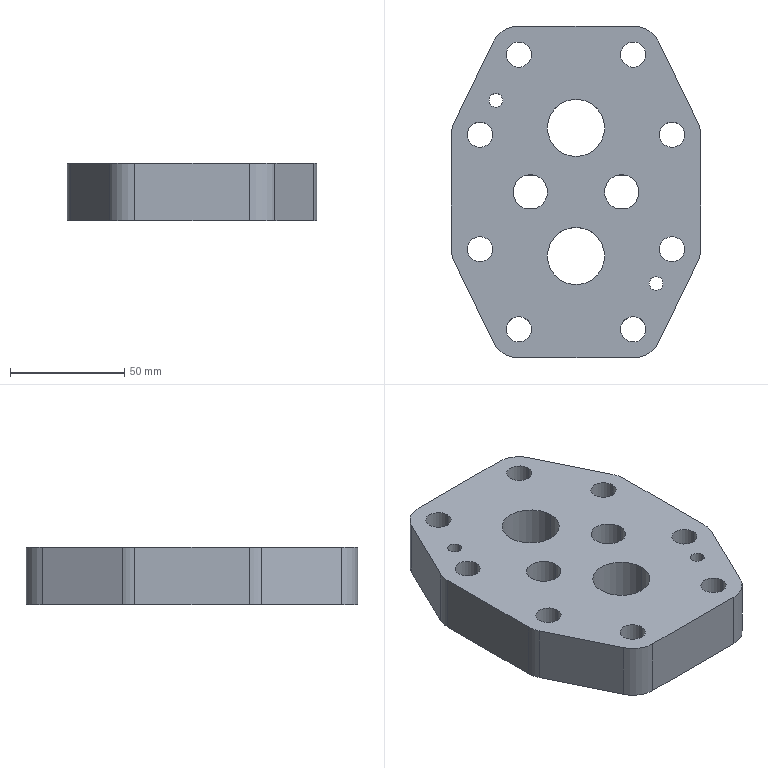Part | SolidWorks | features ICE 3, Extrusion 1, MirrorPattern 1 | 1 solid | 52 faces | box 109 x 145 x 25 mm | volume 291332 mm3 | cylinder 40 | plane 12 | commonest cylinder face diameters 11 x16 25 x12 6 x4 8 x4 15 x4